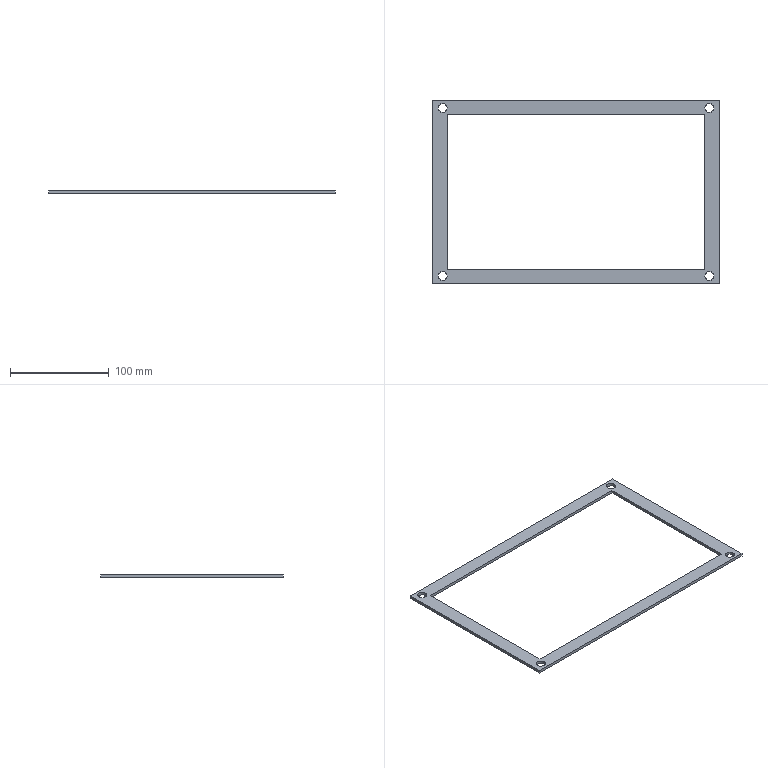Part | SolidWorks | features Extrusion 1, ICE 1, LPattern 1 | 1 solid | 18 faces | box 290 x 185 x 3 mm | volume 37727 mm3 | plane 10 | cylinder 8 | commonest cylinder face diameters 9 x8
STEP:
#1=CARTESIAN_POINT('',(130.5,-85.,0.));
#2=VERTEX_POINT('',#1);
#3=CARTESIAN_POINT('',(139.5,-85.,0.));
#4=VERTEX_POINT('',#3);
#5=CARTESIAN_POINT('',(135.,-85.,0.));
#6=DIRECTION('',(0.,0.,1.));
#7=DIRECTION('',(1.,0.,0.));
#8=AXIS2_PLACEMENT_3D('',#5,#6,#7);
#9=CIRCLE('',#8,4.5);
#10=EDGE_CURVE('',#2,#4,#9,.T.);
#11=ORIENTED_EDGE('',*,*,#10,.F.);
#12=CARTESIAN_POINT('',(130.5,-85.,3.));
#13=VERTEX_POINT('',#12);
#14=CARTESIAN_POINT('',(130.5,-85.,0.));
#15=DIRECTION('',(0.,0.,1.));
#16=VECTOR('',#15,1000.);
#17=LINE('',#14,#16);
#18=EDGE_CURVE('',#2,#13,#17,.T.);
#19=ORIENTED_EDGE('',*,*,#18,.T.);
#20=CARTESIAN_POINT('',(139.5,-85.,3.));
#21=VERTEX_POINT('',#20);
#22=CARTESIAN_POINT('',(135.,-85.,3.));
#23=DIRECTION('',(0.,0.,1.));
#24=DIRECTION('',(1.,0.,0.));
#25=AXIS2_PLACEMENT_3D('',#22,#23,#24);
#26=CIRCLE('',#25,4.5);
#27=EDGE_CURVE('',#13,#21,#26,.T.);
#28=ORIENTED_EDGE('',*,*,#27,.T.);
#29=CARTESIAN_POINT('',(139.5,-85.,0.));
#30=DIRECTION('',(0.,0.,1.));
#31=VECTOR('',#30,1000.);
#32=LINE('',#29,#31);
#33=EDGE_CURVE('',#4,#21,#32,.T.);
#34=ORIENTED_EDGE('',*,*,#33,.F.);
#35=EDGE_LOOP('',(#11,#19,#28,#34));
#36=FACE_OUTER_BOUND('',#35,.T.);
#37=CARTESIAN_POINT('',(135.,-85.,0.));
#38=DIRECTION('',(0.,0.,1.));
#39=DIRECTION('',(1.,0.,0.));
#40=AXIS2_PLACEMENT_3D('',#37,#38,#39);
#41=CYLINDRICAL_SURFACE('',#40,4.5);
#42=ADVANCED_FACE('',(#36),#41,.F.);
#43=CARTESIAN_POINT('',(-139.5,-85.,0.));
#44=VERTEX_POINT('',#43);
#45=CARTESIAN_POINT('',(-130.5,-85.,0.));
#46=VERTEX_POINT('',#45);
#47=CARTESIAN_POINT('',(-135.,-85.,0.));
#48=DIRECTION('',(0.,0.,1.));
#49=DIRECTION('',(1.,0.,0.));
#50=AXIS2_PLACEMENT_3D('',#47,#48,#49);
#51=CIRCLE('',#50,4.5);
#52=EDGE_CURVE('',#44,#46,#51,.T.);
#53=ORIENTED_EDGE('',*,*,#52,.F.);
#54=CARTESIAN_POINT('',(-139.5,-85.,3.));
#55=VERTEX_POINT('',#54);
#56=CARTESIAN_POINT('',(-139.5,-85.,0.));
#57=DIRECTION('',(0.,0.,1.));
#58=VECTOR('',#57,1000.);
#59=LINE('',#56,#58);
#60=EDGE_CURVE('',#44,#55,#59,.T.);
#61=ORIENTED_EDGE('',*,*,#60,.T.);
#62=CARTESIAN_POINT('',(-130.5,-85.,3.));
#63=VERTEX_POINT('',#62);
#64=CARTESIAN_POINT('',(-135.,-85.,3.));
#65=DIRECTION('',(0.,0.,1.));
#66=DIRECTION('',(1.,0.,0.));
#67=AXIS2_PLACEMENT_3D('',#64,#65,#66);
#68=CIRCLE('',#67,4.5);
#69=EDGE_CURVE('',#55,#63,#68,.T.);
#70=ORIENTED_EDGE('',*,*,#69,.T.);
#71=CARTESIAN_POINT('',(-130.5,-85.,0.));
#72=DIRECTION('',(0.,0.,1.));
#73=VECTOR('',#72,1000.);
#74=LINE('',#71,#73);
#75=EDGE_CURVE('',#46,#63,#74,.T.);
#76=ORIENTED_EDGE('',*,*,#75,.F.);
#77=EDGE_LOOP('',(#53,#61,#70,#76));
#78=FACE_OUTER_BOUND('',#77,.T.);
#79=CARTESIAN_POINT('',(-135.,-85.,0.));
#80=DIRECTION('',(0.,0.,1.));
#81=DIRECTION('',(1.,0.,0.));
#82=AXIS2_PLACEMENT_3D('',#79,#80,#81);
#83=CYLINDRICAL_SURFACE('',#82,4.5);
#84=ADVANCED_FACE('',(#78),#83,.F.);
#85=CARTESIAN_POINT('',(130.5,85.,0.));
#86=VERTEX_POINT('',#85);
#87=CARTESIAN_POINT('',(139.5,85.,0.));
#88=VERTEX_POINT('',#87);
#89=CARTESIAN_POINT('',(135.,85.,0.));
#90=DIRECTION('',(0.,0.,1.));
#91=DIRECTION('',(1.,0.,0.));
#92=AXIS2_PLACEMENT_3D('',#89,#90,#91);
#93=CIRCLE('',#92,4.5);
#94=EDGE_CURVE('',#86,#88,#93,.T.);
#95=ORIENTED_EDGE('',*,*,#94,.F.);
#96=CARTESIAN_POINT('',(130.5,85.,3.));
#97=VERTEX_POINT('',#96);
#98=CARTESIAN_POINT('',(130.5,85.,0.));
#99=DIRECTION('',(0.,0.,1.));
#100=VECTOR('',#99,1000.);
#101=LINE('',#98,#100);
#102=EDGE_CURVE('',#86,#97,#101,.T.);
#103=ORIENTED_EDGE('',*,*,#102,.T.);
#104=CARTESIAN_POINT('',(139.5,85.,3.));
#105=VERTEX_POINT('',#104);
#106=CARTESIAN_POINT('',(135.,85.,3.));
#107=DIRECTION('',(0.,0.,1.));
#108=DIRECTION('',(1.,0.,0.));
#109=AXIS2_PLACEMENT_3D('',#106,#107,#108);
#110=CIRCLE('',#109,4.5);
#111=EDGE_CURVE('',#97,#105,#110,.T.);
#112=ORIENTED_EDGE('',*,*,#111,.T.);
#113=CARTESIAN_POINT('',(139.5,85.,0.));
#114=DIRECTION('',(0.,0.,1.));
#115=VECTOR('',#114,1000.);
#116=LINE('',#113,#115);
#117=EDGE_CURVE('',#88,#105,#116,.T.);
#118=ORIENTED_EDGE('',*,*,#117,.F.);
#119=EDGE_LOOP('',(#95,#103,#112,#118));
#120=FACE_OUTER_BOUND('',#119,.T.);
#121=CARTESIAN_POINT('',(135.,85.,0.));
#122=DIRECTION('',(0.,0.,1.));
#123=DIRECTION('',(1.,0.,0.));
#124=AXIS2_PLACEMENT_3D('',#121,#122,#123);
#125=CYLINDRICAL_SURFACE('',#124,4.5);
#126=ADVANCED_FACE('',(#120),#125,.F.);
#127=CARTESIAN_POINT('',(-139.5,85.,0.));
#128=VERTEX_POINT('',#127);
#129=CARTESIAN_POINT('',(-130.5,85.,0.));
#130=VERTEX_POINT('',#129);
#131=CARTESIAN_POINT('',(-135.,85.,0.));
#132=DIRECTION('',(0.,0.,1.));
#133=DIRECTION('',(1.,0.,0.));
#134=AXIS2_PLACEMENT_3D('',#131,#132,#133);
#135=CIRCLE('',#134,4.5);
#136=EDGE_CURVE('',#128,#130,#135,.T.);
#137=ORIENTED_EDGE('',*,*,#136,.F.);
#138=CARTESIAN_POINT('',(-139.5,85.,3.));
#139=VERTEX_POINT('',#138);
#140=CARTESIAN_POINT('',(-139.5,85.,0.));
#141=DIRECTION('',(0.,0.,1.));
#142=VECTOR('',#141,1000.);
#143=LINE('',#140,#142);
#144=EDGE_CURVE('',#128,#139,#143,.T.);
#145=ORIENTED_EDGE('',*,*,#144,.T.);
#146=CARTESIAN_POINT('',(-130.5,85.,3.));
#147=VERTEX_POINT('',#146);
#148=CARTESIAN_POINT('',(-135.,85.,3.));
#149=DIRECTION('',(0.,0.,1.));
#150=DIRECTION('',(1.,0.,0.));
#151=AXIS2_PLACEMENT_3D('',#148,#149,#150);
#152=CIRCLE('',#151,4.5);
#153=EDGE_CURVE('',#139,#147,#152,.T.);
#154=ORIENTED_EDGE('',*,*,#153,.T.);
#155=CARTESIAN_POINT('',(-130.5,85.,0.));
#156=DIRECTION('',(0.,0.,1.));
#157=VECTOR('',#156,1000.);
#158=LINE('',#155,#157);
#159=EDGE_CURVE('',#130,#147,#158,.T.);
#160=ORIENTED_EDGE('',*,*,#159,.F.);
#161=EDGE_LOOP('',(#137,#145,#154,#160));
#162=FACE_OUTER_BOUND('',#161,.T.);
#163=CARTESIAN_POINT('',(-135.,85.,0.));
#164=DIRECTION('',(0.,0.,1.));
#165=DIRECTION('',(1.,0.,0.));
#166=AXIS2_PLACEMENT_3D('',#163,#164,#165);
#167=CYLINDRICAL_SURFACE('',#166,4.5);
#168=ADVANCED_FACE('',(#162),#167,.F.);
#169=CARTESIAN_POINT('',(135.,85.,3.));
#170=DIRECTION('',(0.,0.,1.));
#171=DIRECTION('',(1.,0.,0.));
#172=AXIS2_PLACEMENT_3D('',#169,#170,#171);
#173=CIRCLE('',#172,4.5);
#174=EDGE_CURVE('',#105,#97,#173,.T.);
#175=ORIENTED_EDGE('',*,*,#174,.F.);
#176=ORIENTED_EDGE('',*,*,#111,.F.);
#177=EDGE_LOOP('',(#175,#176));
#178=FACE_BOUND('',#177,.T.);
#179=CARTESIAN_POINT('',(-135.,85.,3.));
#180=DIRECTION('',(0.,0.,1.));
#181=DIRECTION('',(1.,0.,0.));
#182=AXIS2_PLACEMENT_3D('',#179,#180,#181);
#183=CIRCLE('',#182,4.5);
#184=EDGE_CURVE('',#147,#139,#183,.T.);
#185=ORIENTED_EDGE('',*,*,#184,.F.);
#186=ORIENTED_EDGE('',*,*,#153,.F.);
#187=EDGE_LOOP('',(#185,#186));
#188=FACE_BOUND('',#187,.T.);
#189=CARTESIAN_POINT('',(-145.,92.5,3.));
#190=VERTEX_POINT('',#189);
#191=CARTESIAN_POINT('',(-145.,-92.5,3.));
#192=VERTEX_POINT('',#191);
#193=CARTESIAN_POINT('',(-145.,92.5,3.));
#194=DIRECTION('',(0.,-1.,0.));
#195=VECTOR('',#194,1000.);
#196=LINE('',#193,#195);
#197=EDGE_CURVE('',#190,#192,#196,.T.);
#198=ORIENTED_EDGE('',*,*,#197,.T.);
#199=CARTESIAN_POINT('',(145.,-92.5,3.));
#200=VERTEX_POINT('',#199);
#201=CARTESIAN_POINT('',(-145.,-92.5,3.));
#202=DIRECTION('',(1.,0.,0.));
#203=VECTOR('',#202,1000.);
#204=LINE('',#201,#203);
#205=EDGE_CURVE('',#192,#200,#204,.T.);
#206=ORIENTED_EDGE('',*,*,#205,.T.);
#207=CARTESIAN_POINT('',(145.,92.5,3.));
#208=VERTEX_POINT('',#207);
#209=CARTESIAN_POINT('',(145.,92.5,3.));
#210=DIRECTION('',(0.,1.,0.));
#211=VECTOR('',#210,1000.);
#212=LINE('',#209,#211);
#213=EDGE_CURVE('',#200,#208,#212,.T.);
#214=ORIENTED_EDGE('',*,*,#213,.T.);
#215=CARTESIAN_POINT('',(-145.,92.5,3.));
#216=DIRECTION('',(-1.,0.,0.));
#217=VECTOR('',#216,1000.);
#218=LINE('',#215,#217);
#219=EDGE_CURVE('',#208,#190,#218,.T.);
#220=ORIENTED_EDGE('',*,*,#219,.T.);
#221=EDGE_LOOP('',(#198,#206,#214,#220));
#222=FACE_OUTER_BOUND('',#221,.T.);
#223=CARTESIAN_POINT('',(-130.,-78.5,3.));
#224=VERTEX_POINT('',#223);
#225=CARTESIAN_POINT('',(130.,-78.5,3.));
#226=VERTEX_POINT('',#225);
#227=CARTESIAN_POINT('',(-130.,-78.5,3.));
#228=DIRECTION('',(1.,0.,0.));
#229=VECTOR('',#228,1000.);
#230=LINE('',#227,#229);
#231=EDGE_CURVE('',#224,#226,#230,.T.);
#232=ORIENTED_EDGE('',*,*,#231,.F.);
#233=CARTESIAN_POINT('',(-130.,78.5,3.));
#234=VERTEX_POINT('',#233);
#235=CARTESIAN_POINT('',(-130.,78.5,3.));
#236=DIRECTION('',(0.,-1.,0.));
#237=VECTOR('',#236,1000.);
#238=LINE('',#235,#237);
#239=EDGE_CURVE('',#234,#224,#238,.T.);
#240=ORIENTED_EDGE('',*,*,#239,.F.);
#241=CARTESIAN_POINT('',(130.,78.5,3.));
#242=VERTEX_POINT('',#241);
#243=CARTESIAN_POINT('',(-130.,78.5,3.));
#244=DIRECTION('',(-1.,0.,0.));
#245=VECTOR('',#244,1000.);
#246=LINE('',#243,#245);
#247=EDGE_CURVE('',#242,#234,#246,.T.);
#248=ORIENTED_EDGE('',*,*,#247,.F.);
#249=CARTESIAN_POINT('',(130.,78.5,3.));
#250=DIRECTION('',(0.,1.,0.));
#251=VECTOR('',#250,1000.);
#252=LINE('',#249,#251);
#253=EDGE_CURVE('',#226,#242,#252,.T.);
#254=ORIENTED_EDGE('',*,*,#253,.F.);
#255=EDGE_LOOP('',(#232,#240,#248,#254));
#256=FACE_BOUND('',#255,.T.);
#257=CARTESIAN_POINT('',(-135.,-85.,3.));
#258=DIRECTION('',(0.,0.,1.));
#259=DIRECTION('',(1.,0.,0.));
#260=AXIS2_PLACEMENT_3D('',#257,#258,#259);
#261=CIRCLE('',#260,4.5);
#262=EDGE_CURVE('',#63,#55,#261,.T.);
#263=ORIENTED_EDGE('',*,*,#262,.F.);
#264=ORIENTED_EDGE('',*,*,#69,.F.);
#265=EDGE_LOOP('',(#263,#264));
#266=FACE_BOUND('',#265,.T.);
#267=CARTESIAN_POINT('',(135.,-85.,3.));
#268=DIRECTION('',(0.,0.,1.));
#269=DIRECTION('',(1.,0.,0.));
#270=AXIS2_PLACEMENT_3D('',#267,#268,#269);
#271=CIRCLE('',#270,4.5);
#272=EDGE_CURVE('',#21,#13,#271,.T.);
#273=ORIENTED_EDGE('',*,*,#272,.F.);
#274=ORIENTED_EDGE('',*,*,#27,.F.);
#275=EDGE_LOOP('',(#273,#274));
#276=FACE_BOUND('',#275,.T.);
#277=CARTESIAN_POINT('',(0.,0.,3.));
#278=DIRECTION('',(0.,0.,1.));
#279=DIRECTION('',(1.,0.,0.));
#280=AXIS2_PLACEMENT_3D('',#277,#278,#279);
#281=PLANE('',#280);
#282=ADVANCED_FACE('',(#178,#188,#222,#256,#266,#276),#281,.T.);
#283=CARTESIAN_POINT('',(135.,85.,0.));
#284=DIRECTION('',(0.,0.,1.));
#285=DIRECTION('',(1.,0.,0.));
#286=AXIS2_PLACEMENT_3D('',#283,#284,#285);
#287=CIRCLE('',#286,4.5);
#288=EDGE_CURVE('',#88,#86,#287,.T.);
#289=ORIENTED_EDGE('',*,*,#288,.T.);
#290=ORIENTED_EDGE('',*,*,#94,.T.);
#291=EDGE_LOOP('',(#289,#290));
#292=FACE_BOUND('',#291,.T.);
#293=CARTESIAN_POINT('',(-135.,85.,0.));
#294=DIRECTION('',(0.,0.,1.));
#295=DIRECTION('',(1.,0.,0.));
#296=AXIS2_PLACEMENT_3D('',#293,#294,#295);
#297=CIRCLE('',#296,4.5);
#298=EDGE_CURVE('',#130,#128,#297,.T.);
#299=ORIENTED_EDGE('',*,*,#298,.T.);
#300=ORIENTED_EDGE('',*,*,#136,.T.);
#301=EDGE_LOOP('',(#299,#300));
#302=FACE_BOUND('',#301,.T.);
#303=CARTESIAN_POINT('',(-145.,92.5,0.));
#304=VERTEX_POINT('',#303);
#305=CARTESIAN_POINT('',(-145.,-92.5,0.));
#306=VERTEX_POINT('',#305);
#307=CARTESIAN_POINT('',(-145.,92.5,0.));
#308=DIRECTION('',(0.,-1.,0.));
#309=VECTOR('',#308,1000.);
#310=LINE('',#307,#309);
#311=EDGE_CURVE('',#304,#306,#310,.T.);
#312=ORIENTED_EDGE('',*,*,#311,.F.);
#313=CARTESIAN_POINT('',(145.,92.5,0.));
#314=VERTEX_POINT('',#313);
#315=CARTESIAN_POINT('',(-145.,92.5,0.));
#316=DIRECTION('',(-1.,0.,0.));
#317=VECTOR('',#316,1000.);
#318=LINE('',#315,#317);
#319=EDGE_CURVE('',#314,#304,#318,.T.);
#320=ORIENTED_EDGE('',*,*,#319,.F.);
#321=CARTESIAN_POINT('',(145.,-92.5,0.));
#322=VERTEX_POINT('',#321);
#323=CARTESIAN_POINT('',(145.,92.5,0.));
#324=DIRECTION('',(0.,1.,0.));
#325=VECTOR('',#324,1000.);
#326=LINE('',#323,#325);
#327=EDGE_CURVE('',#322,#314,#326,.T.);
#328=ORIENTED_EDGE('',*,*,#327,.F.);
#329=CARTESIAN_POINT('',(-145.,-92.5,0.));
#330=DIRECTION('',(1.,0.,0.));
#331=VECTOR('',#330,1000.);
#332=LINE('',#329,#331);
#333=EDGE_CURVE('',#306,#322,#332,.T.);
#334=ORIENTED_EDGE('',*,*,#333,.F.);
#335=EDGE_LOOP('',(#312,#320,#328,#334));
#336=FACE_OUTER_BOUND('',#335,.T.);
#337=CARTESIAN_POINT('',(-130.,78.5,0.));
#338=VERTEX_POINT('',#337);
#339=CARTESIAN_POINT('',(-130.,-78.5,0.));
#340=VERTEX_POINT('',#339);
#341=CARTESIAN_POINT('',(-130.,78.5,0.));
#342=DIRECTION('',(0.,-1.,0.));
#343=VECTOR('',#342,1000.);
#344=LINE('',#341,#343);
#345=EDGE_CURVE('',#338,#340,#344,.T.);
#346=ORIENTED_EDGE('',*,*,#345,.T.);
#347=CARTESIAN_POINT('',(130.,-78.5,0.));
#348=VERTEX_POINT('',#347);
#349=CARTESIAN_POINT('',(-130.,-78.5,0.));
#350=DIRECTION('',(1.,0.,0.));
#351=VECTOR('',#350,1000.);
#352=LINE('',#349,#351);
#353=EDGE_CURVE('',#340,#348,#352,.T.);
#354=ORIENTED_EDGE('',*,*,#353,.T.);
#355=CARTESIAN_POINT('',(130.,78.5,0.));
#356=VERTEX_POINT('',#355);
#357=CARTESIAN_POINT('',(130.,78.5,0.));
#358=DIRECTION('',(0.,1.,0.));
#359=VECTOR('',#358,1000.);
#360=LINE('',#357,#359);
#361=EDGE_CURVE('',#348,#356,#360,.T.);
#362=ORIENTED_EDGE('',*,*,#361,.T.);
#363=CARTESIAN_POINT('',(-130.,78.5,0.));
#364=DIRECTION('',(-1.,0.,0.));
#365=VECTOR('',#364,1000.);
#366=LINE('',#363,#365);
#367=EDGE_CURVE('',#356,#338,#366,.T.);
#368=ORIENTED_EDGE('',*,*,#367,.T.);
#369=EDGE_LOOP('',(#346,#354,#362,#368));
#370=FACE_BOUND('',#369,.T.);
#371=CARTESIAN_POINT('',(-135.,-85.,0.));
#372=DIRECTION('',(0.,0.,1.));
#373=DIRECTION('',(1.,0.,0.));
#374=AXIS2_PLACEMENT_3D('',#371,#372,#373);
#375=CIRCLE('',#374,4.5);
#376=EDGE_CURVE('',#46,#44,#375,.T.);
#377=ORIENTED_EDGE('',*,*,#376,.T.);
#378=ORIENTED_EDGE('',*,*,#52,.T.);
#379=EDGE_LOOP('',(#377,#378));
#380=FACE_BOUND('',#379,.T.);
#381=CARTESIAN_POINT('',(135.,-85.,0.));
#382=DIRECTION('',(0.,0.,1.));
#383=DIRECTION('',(1.,0.,0.));
#384=AXIS2_PLACEMENT_3D('',#381,#382,#383);
#385=CIRCLE('',#384,4.5);
#386=EDGE_CURVE('',#4,#2,#385,.T.);
#387=ORIENTED_EDGE('',*,*,#386,.T.);
#388=ORIENTED_EDGE('',*,*,#10,.T.);
#389=EDGE_LOOP('',(#387,#388));
#390=FACE_BOUND('',#389,.T.);
#391=CARTESIAN_POINT('',(0.,0.,0.));
#392=DIRECTION('',(0.,0.,1.));
#393=DIRECTION('',(1.,0.,0.));
#394=AXIS2_PLACEMENT_3D('',#391,#392,#393);
#395=PLANE('',#394);
#396=ADVANCED_FACE('',(#292,#302,#336,#370,#380,#390),#395,.F.);
#397=ORIENTED_EDGE('',*,*,#311,.T.);
#398=CARTESIAN_POINT('',(-145.,-92.5,3.));
#399=DIRECTION('',(0.,0.,-1.));
#400=VECTOR('',#399,1000.);
#401=LINE('',#398,#400);
#402=EDGE_CURVE('',#192,#306,#401,.T.);
#403=ORIENTED_EDGE('',*,*,#402,.F.);
#404=ORIENTED_EDGE('',*,*,#197,.F.);
#405=CARTESIAN_POINT('',(-145.,92.5,3.));
#406=DIRECTION('',(0.,0.,-1.));
#407=VECTOR('',#406,1000.);
#408=LINE('',#405,#407);
#409=EDGE_CURVE('',#190,#304,#408,.T.);
#410=ORIENTED_EDGE('',*,*,#409,.T.);
#411=EDGE_LOOP('',(#397,#403,#404,#410));
#412=FACE_OUTER_BOUND('',#411,.T.);
#413=CARTESIAN_POINT('',(-145.,92.5,3.));
#414=DIRECTION('',(1.,0.,0.));
#415=DIRECTION('',(0.,0.,-1.));
#416=AXIS2_PLACEMENT_3D('',#413,#414,#415);
#417=PLANE('',#416);
#418=ADVANCED_FACE('',(#412),#417,.F.);
#419=ORIENTED_EDGE('',*,*,#333,.T.);
#420=CARTESIAN_POINT('',(145.,-92.5,3.));
#421=DIRECTION('',(0.,0.,-1.));
#422=VECTOR('',#421,1000.);
#423=LINE('',#420,#422);
#424=EDGE_CURVE('',#200,#322,#423,.T.);
#425=ORIENTED_EDGE('',*,*,#424,.F.);
#426=ORIENTED_EDGE('',*,*,#205,.F.);
#427=ORIENTED_EDGE('',*,*,#402,.T.);
#428=EDGE_LOOP('',(#419,#425,#426,#427));
#429=FACE_OUTER_BOUND('',#428,.T.);
#430=CARTESIAN_POINT('',(-145.,-92.5,3.));
#431=DIRECTION('',(0.,1.,0.));
#432=DIRECTION('',(-1.,0.,0.));
#433=AXIS2_PLACEMENT_3D('',#430,#431,#432);
#434=PLANE('',#433);
#435=ADVANCED_FACE('',(#429),#434,.F.);
#436=ORIENTED_EDGE('',*,*,#327,.T.);
#437=CARTESIAN_POINT('',(145.,92.5,3.));
#438=DIRECTION('',(0.,0.,-1.));
#439=VECTOR('',#438,1000.);
#440=LINE('',#437,#439);
#441=EDGE_CURVE('',#208,#314,#440,.T.);
#442=ORIENTED_EDGE('',*,*,#441,.F.);
#443=ORIENTED_EDGE('',*,*,#213,.F.);
#444=ORIENTED_EDGE('',*,*,#424,.T.);
#445=EDGE_LOOP('',(#436,#442,#443,#444));
#446=FACE_OUTER_BOUND('',#445,.T.);
#447=CARTESIAN_POINT('',(145.,92.5,3.));
#448=DIRECTION('',(-1.,0.,0.));
#449=DIRECTION('',(0.,-1.,0.));
#450=AXIS2_PLACEMENT_3D('',#447,#448,#449);
#451=PLANE('',#450);
#452=ADVANCED_FACE('',(#446),#451,.F.);
#453=ORIENTED_EDGE('',*,*,#319,.T.);
#454=ORIENTED_EDGE('',*,*,#409,.F.);
#455=ORIENTED_EDGE('',*,*,#219,.F.);
#456=ORIENTED_EDGE('',*,*,#441,.T.);
#457=EDGE_LOOP('',(#453,#454,#455,#456));
#458=FACE_OUTER_BOUND('',#457,.T.);
#459=CARTESIAN_POINT('',(-145.,92.5,3.));
#460=DIRECTION('',(0.,-1.,0.));
#461=DIRECTION('',(0.,0.,-1.));
#462=AXIS2_PLACEMENT_3D('',#459,#460,#461);
#463=PLANE('',#462);
#464=ADVANCED_FACE('',(#458),#463,.F.);
#465=ORIENTED_EDGE('',*,*,#345,.F.);
#466=CARTESIAN_POINT('',(-130.,78.5,3.));
#467=DIRECTION('',(0.,0.,-1.));
#468=VECTOR('',#467,1000.);
#469=LINE('',#466,#468);
#470=EDGE_CURVE('',#234,#338,#469,.T.);
#471=ORIENTED_EDGE('',*,*,#470,.F.);
#472=ORIENTED_EDGE('',*,*,#239,.T.);
#473=CARTESIAN_POINT('',(-130.,-78.5,3.));
#474=DIRECTION('',(0.,0.,-1.));
#475=VECTOR('',#474,1000.);
#476=LINE('',#473,#475);
#477=EDGE_CURVE('',#224,#340,#476,.T.);
#478=ORIENTED_EDGE('',*,*,#477,.T.);
#479=EDGE_LOOP('',(#465,#471,#472,#478));
#480=FACE_OUTER_BOUND('',#479,.T.);
#481=CARTESIAN_POINT('',(-130.,78.5,3.));
#482=DIRECTION('',(1.,0.,0.));
#483=DIRECTION('',(0.,0.,-1.));
#484=AXIS2_PLACEMENT_3D('',#481,#482,#483);
#485=PLANE('',#484);
#486=ADVANCED_FACE('',(#480),#485,.T.);
#487=ORIENTED_EDGE('',*,*,#353,.F.);
#488=ORIENTED_EDGE('',*,*,#477,.F.);
#489=ORIENTED_EDGE('',*,*,#231,.T.);
#490=CARTESIAN_POINT('',(130.,-78.5,3.));
#491=DIRECTION('',(0.,0.,-1.));
#492=VECTOR('',#491,1000.);
#493=LINE('',#490,#492);
#494=EDGE_CURVE('',#226,#348,#493,.T.);
#495=ORIENTED_EDGE('',*,*,#494,.T.);
#496=EDGE_LOOP('',(#487,#488,#489,#495));
#497=FACE_OUTER_BOUND('',#496,.T.);
#498=CARTESIAN_POINT('',(-130.,-78.5,3.));
#499=DIRECTION('',(0.,1.,0.));
#500=DIRECTION('',(0.,0.,1.));
#501=AXIS2_PLACEMENT_3D('',#498,#499,#500);
#502=PLANE('',#501);
#503=ADVANCED_FACE('',(#497),#502,.T.);
#504=ORIENTED_EDGE('',*,*,#361,.F.);
#505=ORIENTED_EDGE('',*,*,#494,.F.);
#506=ORIENTED_EDGE('',*,*,#253,.T.);
#507=CARTESIAN_POINT('',(130.,78.5,3.));
#508=DIRECTION('',(0.,0.,-1.));
#509=VECTOR('',#508,1000.);
#510=LINE('',#507,#509);
#511=EDGE_CURVE('',#242,#356,#510,.T.);
#512=ORIENTED_EDGE('',*,*,#511,.T.);
#513=EDGE_LOOP('',(#504,#505,#506,#512));
#514=FACE_OUTER_BOUND('',#513,.T.);
#515=CARTESIAN_POINT('',(130.,78.5,3.));
#516=DIRECTION('',(-1.,0.,0.));
#517=DIRECTION('',(0.,0.,1.));
#518=AXIS2_PLACEMENT_3D('',#515,#516,#517);
#519=PLANE('',#518);
#520=ADVANCED_FACE('',(#514),#519,.T.);
#521=ORIENTED_EDGE('',*,*,#367,.F.);
#522=ORIENTED_EDGE('',*,*,#511,.F.);
#523=ORIENTED_EDGE('',*,*,#247,.T.);
#524=ORIENTED_EDGE('',*,*,#470,.T.);
#525=EDGE_LOOP('',(#521,#522,#523,#524));
#526=FACE_OUTER_BOUND('',#525,.T.);
#527=CARTESIAN_POINT('',(-130.,78.5,3.));
#528=DIRECTION('',(0.,-1.,0.));
#529=DIRECTION('',(0.,0.,-1.));
#530=AXIS2_PLACEMENT_3D('',#527,#528,#529);
#531=PLANE('',#530);
#532=ADVANCED_FACE('',(#526),#531,.T.);
#533=ORIENTED_EDGE('',*,*,#144,.F.);
#534=ORIENTED_EDGE('',*,*,#298,.F.);
#535=ORIENTED_EDGE('',*,*,#159,.T.);
#536=ORIENTED_EDGE('',*,*,#184,.T.);
#537=EDGE_LOOP('',(#533,#534,#535,#536));
#538=FACE_OUTER_BOUND('',#537,.T.);
#539=CARTESIAN_POINT('',(-135.,85.,0.));
#540=DIRECTION('',(0.,0.,1.));
#541=DIRECTION('',(1.,0.,0.));
#542=AXIS2_PLACEMENT_3D('',#539,#540,#541);
#543=CYLINDRICAL_SURFACE('',#542,4.5);
#544=ADVANCED_FACE('',(#538),#543,.F.);
#545=ORIENTED_EDGE('',*,*,#102,.F.);
#546=ORIENTED_EDGE('',*,*,#288,.F.);
#547=ORIENTED_EDGE('',*,*,#117,.T.);
#548=ORIENTED_EDGE('',*,*,#174,.T.);
#549=EDGE_LOOP('',(#545,#546,#547,#548));
#550=FACE_OUTER_BOUND('',#549,.T.);
#551=CARTESIAN_POINT('',(135.,85.,0.));
#552=DIRECTION('',(0.,0.,1.));
#553=DIRECTION('',(1.,0.,0.));
#554=AXIS2_PLACEMENT_3D('',#551,#552,#553);
#555=CYLINDRICAL_SURFACE('',#554,4.5);
#556=ADVANCED_FACE('',(#550),#555,.F.);
#557=ORIENTED_EDGE('',*,*,#60,.F.);
#558=ORIENTED_EDGE('',*,*,#376,.F.);
#559=ORIENTED_EDGE('',*,*,#75,.T.);
#560=ORIENTED_EDGE('',*,*,#262,.T.);
#561=EDGE_LOOP('',(#557,#558,#559,#560));
#562=FACE_OUTER_BOUND('',#561,.T.);
#563=CARTESIAN_POINT('',(-135.,-85.,0.));
#564=DIRECTION('',(0.,0.,1.));
#565=DIRECTION('',(1.,0.,0.));
#566=AXIS2_PLACEMENT_3D('',#563,#564,#565);
#567=CYLINDRICAL_SURFACE('',#566,4.5);
#568=ADVANCED_FACE('',(#562),#567,.F.);
#569=ORIENTED_EDGE('',*,*,#18,.F.);
#570=ORIENTED_EDGE('',*,*,#386,.F.);
#571=ORIENTED_EDGE('',*,*,#33,.T.);
#572=ORIENTED_EDGE('',*,*,#272,.T.);
#573=EDGE_LOOP('',(#569,#570,#571,#572));
#574=FACE_OUTER_BOUND('',#573,.T.);
#575=CARTESIAN_POINT('',(135.,-85.,0.));
#576=DIRECTION('',(0.,0.,1.));
#577=DIRECTION('',(1.,0.,0.));
#578=AXIS2_PLACEMENT_3D('',#575,#576,#577);
#579=CYLINDRICAL_SURFACE('',#578,4.5);
#580=ADVANCED_FACE('',(#574),#579,.F.);
#581=CLOSED_SHELL('',(#42,#84,#126,#168,#282,#396,#418,#435,#452,#464,#486,#503,#520,#532,#544,#556,#568,#580));
#582=MANIFOLD_SOLID_BREP('',#581);
#583=CARTESIAN_POINT('',(0.,0.,0.));
#584=DIRECTION('',(0.,0.,1.));
#585=DIRECTION('',(1.,0.,0.));
#586=AXIS2_PLACEMENT_3D('',#583,#584,#585);
#587=(LENGTH_UNIT()NAMED_UNIT(*)SI_UNIT(.MILLI.,.METRE.));
#588=UNCERTAINTY_MEASURE_WITH_UNIT(LENGTH_MEASURE(0.00001),#587,'','');
#589=(NAMED_UNIT(*)PLANE_ANGLE_UNIT()SI_UNIT($,.RADIAN.));
#590=(NAMED_UNIT(*)SI_UNIT($,.STERADIAN.)SOLID_ANGLE_UNIT());
#591=(GEOMETRIC_REPRESENTATION_CONTEXT(3)GLOBAL_UNCERTAINTY_ASSIGNED_CONTEXT((#588))GLOBAL_UNIT_ASSIGNED_CONTEXT((#587,#589,#590))REPRESENTATION_CONTEXT('',''));
#592=ADVANCED_BREP_SHAPE_REPRESENTATION('',(#582,#586),#591);